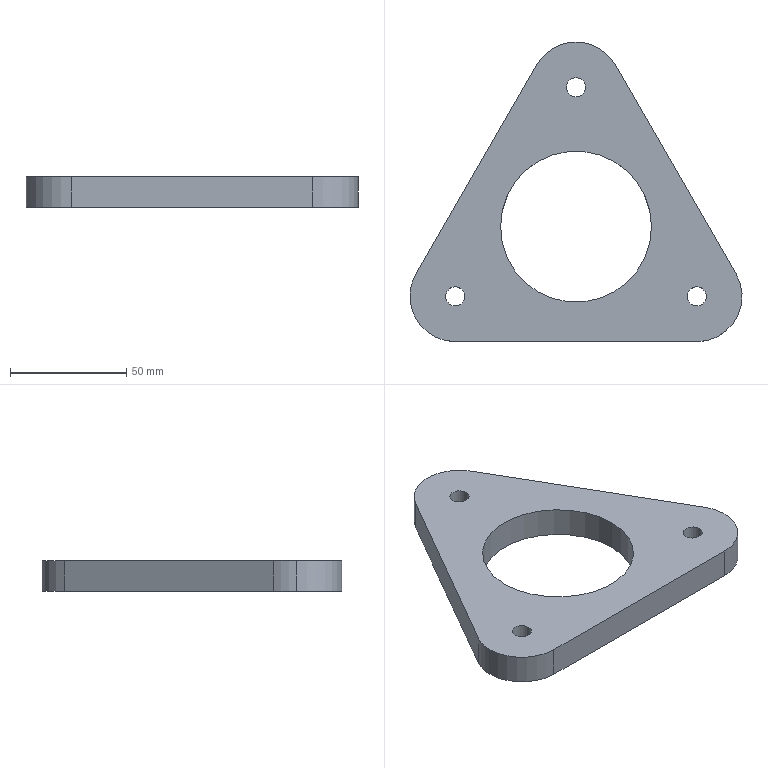Part | SolidWorks | features Extrusion 1, ICE 1, Scale 1 | 1 solid | 36 faces | box 143 x 129.067 x 13 mm | volume 109293 mm3 | cylinder 22 | plane 14 | commonest cylinder face diameters 8.255 x6 11.7 x6 2.6 x4 39 x4 65 x2
STEP:
#1=CARTESIAN_POINT('',(56.847,-26.746,3.9));
#2=VERTEX_POINT('',#1);
#3=CARTESIAN_POINT('',(46.15,-30.022,3.9));
#4=VERTEX_POINT('',#3);
#5=CARTESIAN_POINT('',(52.,-30.022,3.9));
#6=DIRECTION('',(0.,0.,1.));
#7=DIRECTION('',(1.,0.,0.));
#8=AXIS2_PLACEMENT_3D('',#5,#6,#7);
#9=CIRCLE('',#8,5.85);
#10=EDGE_CURVE('',#2,#4,#9,.T.);
#11=ORIENTED_EDGE('',*,*,#10,.T.);
#12=CARTESIAN_POINT('',(46.15,-30.022,0.));
#13=VERTEX_POINT('',#12);
#14=CARTESIAN_POINT('',(46.15,-30.022,3.9));
#15=DIRECTION('',(0.,0.,-1.));
#16=VECTOR('',#15,1000.);
#17=LINE('',#14,#16);
#18=EDGE_CURVE('',#4,#13,#17,.T.);
#19=ORIENTED_EDGE('',*,*,#18,.T.);
#20=CARTESIAN_POINT('',(56.847,-26.746,0.));
#21=VERTEX_POINT('',#20);
#22=CARTESIAN_POINT('',(52.,-30.022,0.));
#23=DIRECTION('',(0.,0.,1.));
#24=DIRECTION('',(1.,0.,0.));
#25=AXIS2_PLACEMENT_3D('',#22,#23,#24);
#26=CIRCLE('',#25,5.85);
#27=EDGE_CURVE('',#21,#13,#26,.T.);
#28=ORIENTED_EDGE('',*,*,#27,.F.);
#29=CARTESIAN_POINT('',(56.847,-26.746,3.9));
#30=DIRECTION('',(0.,0.,-1.));
#31=VECTOR('',#30,1000.);
#32=LINE('',#29,#31);
#33=EDGE_CURVE('',#2,#21,#32,.T.);
#34=ORIENTED_EDGE('',*,*,#33,.F.);
#35=EDGE_LOOP('',(#11,#19,#28,#34));
#36=FACE_OUTER_BOUND('',#35,.T.);
#37=CARTESIAN_POINT('',(52.,-30.022,3.9));
#38=DIRECTION('',(0.,0.,-1.));
#39=DIRECTION('',(-1.,0.,0.));
#40=AXIS2_PLACEMENT_3D('',#37,#38,#39);
#41=CYLINDRICAL_SURFACE('',#40,5.85);
#42=ADVANCED_FACE('',(#36),#41,.F.);
#43=CARTESIAN_POINT('',(-5.85,60.044,3.9));
#44=VERTEX_POINT('',#43);
#45=CARTESIAN_POINT('',(5.85,60.044,3.9));
#46=VERTEX_POINT('',#45);
#47=CARTESIAN_POINT('',(0.,60.044,3.9));
#48=DIRECTION('',(0.,0.,1.));
#49=DIRECTION('',(1.,0.,0.));
#50=AXIS2_PLACEMENT_3D('',#47,#48,#49);
#51=CIRCLE('',#50,5.85);
#52=EDGE_CURVE('',#44,#46,#51,.T.);
#53=ORIENTED_EDGE('',*,*,#52,.T.);
#54=CARTESIAN_POINT('',(5.85,60.044,0.));
#55=VERTEX_POINT('',#54);
#56=CARTESIAN_POINT('',(5.85,60.044,3.9));
#57=DIRECTION('',(0.,0.,-1.));
#58=VECTOR('',#57,1000.);
#59=LINE('',#56,#58);
#60=EDGE_CURVE('',#46,#55,#59,.T.);
#61=ORIENTED_EDGE('',*,*,#60,.T.);
#62=CARTESIAN_POINT('',(-5.85,60.044,0.));
#63=VERTEX_POINT('',#62);
#64=CARTESIAN_POINT('',(0.,60.044,0.));
#65=DIRECTION('',(0.,0.,1.));
#66=DIRECTION('',(1.,0.,0.));
#67=AXIS2_PLACEMENT_3D('',#64,#65,#66);
#68=CIRCLE('',#67,5.85);
#69=EDGE_CURVE('',#63,#55,#68,.T.);
#70=ORIENTED_EDGE('',*,*,#69,.F.);
#71=CARTESIAN_POINT('',(-5.85,60.044,3.9));
#72=DIRECTION('',(0.,0.,-1.));
#73=VECTOR('',#72,1000.);
#74=LINE('',#71,#73);
#75=EDGE_CURVE('',#44,#63,#74,.T.);
#76=ORIENTED_EDGE('',*,*,#75,.F.);
#77=EDGE_LOOP('',(#53,#61,#70,#76));
#78=FACE_OUTER_BOUND('',#77,.T.);
#79=CARTESIAN_POINT('',(0.,60.044,3.9));
#80=DIRECTION('',(0.,0.,-1.));
#81=DIRECTION('',(-1.,0.,0.));
#82=AXIS2_PLACEMENT_3D('',#79,#80,#81);
#83=CYLINDRICAL_SURFACE('',#82,5.85);
#84=ADVANCED_FACE('',(#78),#83,.F.);
#85=CARTESIAN_POINT('',(-5.26,62.604,3.9));
#86=VERTEX_POINT('',#85);
#87=CARTESIAN_POINT('',(0.,60.044,3.9));
#88=DIRECTION('',(0.,0.,1.));
#89=DIRECTION('',(1.,0.,0.));
#90=AXIS2_PLACEMENT_3D('',#87,#88,#89);
#91=CIRCLE('',#90,5.85);
#92=EDGE_CURVE('',#86,#44,#91,.T.);
#93=ORIENTED_EDGE('',*,*,#92,.T.);
#94=ORIENTED_EDGE('',*,*,#75,.T.);
#95=CARTESIAN_POINT('',(-5.26,62.604,0.));
#96=VERTEX_POINT('',#95);
#97=CARTESIAN_POINT('',(0.,60.044,0.));
#98=DIRECTION('',(0.,0.,1.));
#99=DIRECTION('',(1.,0.,0.));
#100=AXIS2_PLACEMENT_3D('',#97,#98,#99);
#101=CIRCLE('',#100,5.85);
#102=EDGE_CURVE('',#96,#63,#101,.T.);
#103=ORIENTED_EDGE('',*,*,#102,.F.);
#104=CARTESIAN_POINT('',(-5.26,62.604,3.9));
#105=DIRECTION('',(0.,0.,-1.));
#106=VECTOR('',#105,1000.);
#107=LINE('',#104,#106);
#108=EDGE_CURVE('',#86,#96,#107,.T.);
#109=ORIENTED_EDGE('',*,*,#108,.F.);
#110=EDGE_LOOP('',(#93,#94,#103,#109));
#111=FACE_OUTER_BOUND('',#110,.T.);
#112=CARTESIAN_POINT('',(0.,60.044,3.9));
#113=DIRECTION('',(0.,0.,-1.));
#114=DIRECTION('',(-1.,0.,0.));
#115=AXIS2_PLACEMENT_3D('',#112,#113,#114);
#116=CYLINDRICAL_SURFACE('',#115,5.85);
#117=ADVANCED_FACE('',(#111),#116,.F.);
#118=CARTESIAN_POINT('',(-62.084,-34.494,3.9));
#119=VERTEX_POINT('',#118);
#120=CARTESIAN_POINT('',(-62.307,-35.222,3.9));
#121=VERTEX_POINT('',#120);
#122=CARTESIAN_POINT('',(-61.007,-35.222,3.9));
#123=DIRECTION('',(0.,0.,1.));
#124=DIRECTION('',(1.,0.,0.));
#125=AXIS2_PLACEMENT_3D('',#122,#123,#124);
#126=CIRCLE('',#125,1.3);
#127=EDGE_CURVE('',#119,#121,#126,.T.);
#128=ORIENTED_EDGE('',*,*,#127,.T.);
#129=CARTESIAN_POINT('',(-62.307,-35.222,0.));
#130=VERTEX_POINT('',#129);
#131=CARTESIAN_POINT('',(-62.307,-35.222,3.9));
#132=DIRECTION('',(0.,0.,-1.));
#133=VECTOR('',#132,1000.);
#134=LINE('',#131,#133);
#135=EDGE_CURVE('',#121,#130,#134,.T.);
#136=ORIENTED_EDGE('',*,*,#135,.T.);
#137=CARTESIAN_POINT('',(-62.084,-34.494,0.));
#138=VERTEX_POINT('',#137);
#139=CARTESIAN_POINT('',(-61.007,-35.222,0.));
#140=DIRECTION('',(0.,0.,1.));
#141=DIRECTION('',(1.,0.,0.));
#142=AXIS2_PLACEMENT_3D('',#139,#140,#141);
#143=CIRCLE('',#142,1.3);
#144=EDGE_CURVE('',#138,#130,#143,.T.);
#145=ORIENTED_EDGE('',*,*,#144,.F.);
#146=CARTESIAN_POINT('',(-62.084,-34.494,3.9));
#147=DIRECTION('',(0.,0.,-1.));
#148=VECTOR('',#147,1000.);
#149=LINE('',#146,#148);
#150=EDGE_CURVE('',#119,#138,#149,.T.);
#151=ORIENTED_EDGE('',*,*,#150,.F.);
#152=EDGE_LOOP('',(#128,#136,#145,#151));
#153=FACE_OUTER_BOUND('',#152,.T.);
#154=CARTESIAN_POINT('',(-61.007,-35.222,3.9));
#155=DIRECTION('',(0.,0.,-1.));
#156=DIRECTION('',(-1.,0.,0.));
#157=AXIS2_PLACEMENT_3D('',#154,#155,#156);
#158=CYLINDRICAL_SURFACE('',#157,1.3);
#159=ADVANCED_FACE('',(#153),#158,.F.);
#160=CARTESIAN_POINT('',(-32.5,0.,13.));
#161=VERTEX_POINT('',#160);
#162=CARTESIAN_POINT('',(32.5,0.,13.));
#163=VERTEX_POINT('',#162);
#164=CARTESIAN_POINT('',(0.,0.,13.));
#165=DIRECTION('',(0.,0.,1.));
#166=DIRECTION('',(1.,0.,0.));
#167=AXIS2_PLACEMENT_3D('',#164,#165,#166);
#168=CIRCLE('',#167,32.5);
#169=EDGE_CURVE('',#161,#163,#168,.T.);
#170=ORIENTED_EDGE('',*,*,#169,.T.);
#171=CARTESIAN_POINT('',(32.5,0.,0.));
#172=VERTEX_POINT('',#171);
#173=CARTESIAN_POINT('',(32.5,0.,13.));
#174=DIRECTION('',(0.,0.,-1.));
#175=VECTOR('',#174,1000.);
#176=LINE('',#173,#175);
#177=EDGE_CURVE('',#163,#172,#176,.T.);
#178=ORIENTED_EDGE('',*,*,#177,.T.);
#179=CARTESIAN_POINT('',(-32.5,0.,0.));
#180=VERTEX_POINT('',#179);
#181=CARTESIAN_POINT('',(0.,0.,0.));
#182=DIRECTION('',(0.,0.,1.));
#183=DIRECTION('',(1.,0.,0.));
#184=AXIS2_PLACEMENT_3D('',#181,#182,#183);
#185=CIRCLE('',#184,32.5);
#186=EDGE_CURVE('',#180,#172,#185,.T.);
#187=ORIENTED_EDGE('',*,*,#186,.F.);
#188=CARTESIAN_POINT('',(-32.5,0.,13.));
#189=DIRECTION('',(0.,0.,-1.));
#190=VECTOR('',#189,1000.);
#191=LINE('',#188,#190);
#192=EDGE_CURVE('',#161,#180,#191,.T.);
#193=ORIENTED_EDGE('',*,*,#192,.F.);
#194=EDGE_LOOP('',(#170,#178,#187,#193));
#195=FACE_OUTER_BOUND('',#194,.T.);
#196=CARTESIAN_POINT('',(0.,0.,13.));
#197=DIRECTION('',(0.,0.,-1.));
#198=DIRECTION('',(-1.,0.,0.));
#199=AXIS2_PLACEMENT_3D('',#196,#197,#198);
#200=CYLINDRICAL_SURFACE('',#199,32.5);
#201=ADVANCED_FACE('',(#195),#200,.F.);
#202=CARTESIAN_POINT('',(-4.127,60.044,13.));
#203=VERTEX_POINT('',#202);
#204=CARTESIAN_POINT('',(4.127,60.044,13.));
#205=VERTEX_POINT('',#204);
#206=CARTESIAN_POINT('',(0.,60.044,13.));
#207=DIRECTION('',(0.,0.,1.));
#208=DIRECTION('',(1.,0.,0.));
#209=AXIS2_PLACEMENT_3D('',#206,#207,#208);
#210=CIRCLE('',#209,4.127);
#211=EDGE_CURVE('',#203,#205,#210,.T.);
#212=ORIENTED_EDGE('',*,*,#211,.T.);
#213=CARTESIAN_POINT('',(4.128,60.044,3.9));
#214=VERTEX_POINT('',#213);
#215=CARTESIAN_POINT('',(4.127,60.044,13.));
#216=DIRECTION('',(0.,0.,-1.));
#217=VECTOR('',#216,1000.);
#218=LINE('',#215,#217);
#219=EDGE_CURVE('',#205,#214,#218,.T.);
#220=ORIENTED_EDGE('',*,*,#219,.T.);
#221=CARTESIAN_POINT('',(-4.127,60.044,3.9));
#222=VERTEX_POINT('',#221);
#223=CARTESIAN_POINT('',(0.,60.044,3.9));
#224=DIRECTION('',(0.,0.,1.));
#225=DIRECTION('',(1.,0.,0.));
#226=AXIS2_PLACEMENT_3D('',#223,#224,#225);
#227=CIRCLE('',#226,4.127);
#228=EDGE_CURVE('',#222,#214,#227,.T.);
#229=ORIENTED_EDGE('',*,*,#228,.F.);
#230=CARTESIAN_POINT('',(-4.127,60.044,13.));
#231=DIRECTION('',(0.,0.,-1.));
#232=VECTOR('',#231,1000.);
#233=LINE('',#230,#232);
#234=EDGE_CURVE('',#203,#222,#233,.T.);
#235=ORIENTED_EDGE('',*,*,#234,.F.);
#236=EDGE_LOOP('',(#212,#220,#229,#235));
#237=FACE_OUTER_BOUND('',#236,.T.);
#238=CARTESIAN_POINT('',(0.,60.044,13.));
#239=DIRECTION('',(0.,0.,-1.));
#240=DIRECTION('',(-1.,0.,0.));
#241=AXIS2_PLACEMENT_3D('',#238,#239,#240);
#242=CYLINDRICAL_SURFACE('',#241,4.127);
#243=ADVANCED_FACE('',(#237),#242,.F.);
#244=CARTESIAN_POINT('',(47.873,-30.022,13.));
#245=VERTEX_POINT('',#244);
#246=CARTESIAN_POINT('',(56.128,-30.022,13.));
#247=VERTEX_POINT('',#246);
#248=CARTESIAN_POINT('',(52.,-30.022,13.));
#249=DIRECTION('',(0.,0.,1.));
#250=DIRECTION('',(1.,0.,0.));
#251=AXIS2_PLACEMENT_3D('',#248,#249,#250);
#252=CIRCLE('',#251,4.127);
#253=EDGE_CURVE('',#245,#247,#252,.T.);
#254=ORIENTED_EDGE('',*,*,#253,.T.);
#255=CARTESIAN_POINT('',(56.127,-30.022,3.9));
#256=VERTEX_POINT('',#255);
#257=CARTESIAN_POINT('',(56.128,-30.022,13.));
#258=DIRECTION('',(0.,0.,-1.));
#259=VECTOR('',#258,1000.);
#260=LINE('',#257,#259);
#261=EDGE_CURVE('',#247,#256,#260,.T.);
#262=ORIENTED_EDGE('',*,*,#261,.T.);
#263=CARTESIAN_POINT('',(47.872,-30.022,3.9));
#264=VERTEX_POINT('',#263);
#265=CARTESIAN_POINT('',(52.,-30.022,3.9));
#266=DIRECTION('',(0.,0.,1.));
#267=DIRECTION('',(1.,0.,0.));
#268=AXIS2_PLACEMENT_3D('',#265,#266,#267);
#269=CIRCLE('',#268,4.127);
#270=EDGE_CURVE('',#264,#256,#269,.T.);
#271=ORIENTED_EDGE('',*,*,#270,.F.);
#272=CARTESIAN_POINT('',(47.873,-30.022,13.));
#273=DIRECTION('',(0.,0.,-1.));
#274=VECTOR('',#273,1000.);
#275=LINE('',#272,#274);
#276=EDGE_CURVE('',#245,#264,#275,.T.);
#277=ORIENTED_EDGE('',*,*,#276,.F.);
#278=EDGE_LOOP('',(#254,#262,#271,#277));
#279=FACE_OUTER_BOUND('',#278,.T.);
#280=CARTESIAN_POINT('',(52.,-30.022,13.));
#281=DIRECTION('',(0.,0.,-1.));
#282=DIRECTION('',(-1.,0.,0.));
#283=AXIS2_PLACEMENT_3D('',#280,#281,#282);
#284=CYLINDRICAL_SURFACE('',#283,4.127);
#285=ADVANCED_FACE('',(#279),#284,.F.);
#286=CARTESIAN_POINT('',(-56.127,-30.022,13.));
#287=VERTEX_POINT('',#286);
#288=CARTESIAN_POINT('',(-47.872,-30.022,13.));
#289=VERTEX_POINT('',#288);
#290=CARTESIAN_POINT('',(-52.,-30.022,13.));
#291=DIRECTION('',(0.,0.,1.));
#292=DIRECTION('',(1.,0.,0.));
#293=AXIS2_PLACEMENT_3D('',#290,#291,#292);
#294=CIRCLE('',#293,4.127);
#295=EDGE_CURVE('',#287,#289,#294,.T.);
#296=ORIENTED_EDGE('',*,*,#295,.T.);
#297=CARTESIAN_POINT('',(-47.872,-30.022,3.9));
#298=VERTEX_POINT('',#297);
#299=CARTESIAN_POINT('',(-47.872,-30.022,13.));
#300=DIRECTION('',(0.,0.,-1.));
#301=VECTOR('',#300,1000.);
#302=LINE('',#299,#301);
#303=EDGE_CURVE('',#289,#298,#302,.T.);
#304=ORIENTED_EDGE('',*,*,#303,.T.);
#305=CARTESIAN_POINT('',(-56.127,-30.022,3.9));
#306=VERTEX_POINT('',#305);
#307=CARTESIAN_POINT('',(-52.,-30.022,3.9));
#308=DIRECTION('',(0.,0.,1.));
#309=DIRECTION('',(1.,0.,0.));
#310=AXIS2_PLACEMENT_3D('',#307,#308,#309);
#311=CIRCLE('',#310,4.127);
#312=EDGE_CURVE('',#306,#298,#311,.T.);
#313=ORIENTED_EDGE('',*,*,#312,.F.);
#314=CARTESIAN_POINT('',(-56.127,-30.022,13.));
#315=DIRECTION('',(0.,0.,-1.));
#316=VECTOR('',#315,1000.);
#317=LINE('',#314,#316);
#318=EDGE_CURVE('',#287,#306,#317,.T.);
#319=ORIENTED_EDGE('',*,*,#318,.F.);
#320=EDGE_LOOP('',(#296,#304,#313,#319));
#321=FACE_OUTER_BOUND('',#320,.T.);
#322=CARTESIAN_POINT('',(-52.,-30.022,13.));
#323=DIRECTION('',(0.,0.,-1.));
#324=DIRECTION('',(-1.,0.,0.));
#325=AXIS2_PLACEMENT_3D('',#322,#323,#324);
#326=CYLINDRICAL_SURFACE('',#325,4.127);
#327=ADVANCED_FACE('',(#321),#326,.F.);
#328=CARTESIAN_POINT('',(-71.5,-30.022,13.));
#329=VERTEX_POINT('',#328);
#330=CARTESIAN_POINT('',(-52.,-49.522,13.));
#331=VERTEX_POINT('',#330);
#332=CARTESIAN_POINT('',(-52.,-30.022,13.));
#333=DIRECTION('',(0.,0.,1.));
#334=DIRECTION('',(1.,0.,0.));
#335=AXIS2_PLACEMENT_3D('',#332,#333,#334);
#336=CIRCLE('',#335,19.5);
#337=EDGE_CURVE('',#329,#331,#336,.T.);
#338=ORIENTED_EDGE('',*,*,#337,.F.);
#339=CARTESIAN_POINT('',(-71.5,-30.022,0.));
#340=VERTEX_POINT('',#339);
#341=CARTESIAN_POINT('',(-71.5,-30.022,13.));
#342=DIRECTION('',(0.,0.,-1.));
#343=VECTOR('',#342,1000.);
#344=LINE('',#341,#343);
#345=EDGE_CURVE('',#329,#340,#344,.T.);
#346=ORIENTED_EDGE('',*,*,#345,.T.);
#347=CARTESIAN_POINT('',(-52.,-49.522,0.));
#348=VERTEX_POINT('',#347);
#349=CARTESIAN_POINT('',(-52.,-30.022,0.));
#350=DIRECTION('',(0.,0.,1.));
#351=DIRECTION('',(1.,0.,0.));
#352=AXIS2_PLACEMENT_3D('',#349,#350,#351);
#353=CIRCLE('',#352,19.5);
#354=EDGE_CURVE('',#340,#348,#353,.T.);
#355=ORIENTED_EDGE('',*,*,#354,.T.);
#356=CARTESIAN_POINT('',(-52.,-49.522,13.));
#357=DIRECTION('',(0.,0.,-1.));
#358=VECTOR('',#357,1000.);
#359=LINE('',#356,#358);
#360=EDGE_CURVE('',#331,#348,#359,.T.);
#361=ORIENTED_EDGE('',*,*,#360,.F.);
#362=EDGE_LOOP('',(#338,#346,#355,#361));
#363=FACE_OUTER_BOUND('',#362,.T.);
#364=CARTESIAN_POINT('',(-52.,-30.022,13.));
#365=DIRECTION('',(0.,0.,-1.));
#366=DIRECTION('',(-1.,0.,0.));
#367=AXIS2_PLACEMENT_3D('',#364,#365,#366);
#368=CYLINDRICAL_SURFACE('',#367,19.5);
#369=ADVANCED_FACE('',(#363),#368,.T.);
#370=ORIENTED_EDGE('',*,*,#102,.T.);
#371=ORIENTED_EDGE('',*,*,#69,.T.);
#372=CARTESIAN_POINT('',(5.26,62.604,0.));
#373=VERTEX_POINT('',#372);
#374=CARTESIAN_POINT('',(0.,60.044,0.));
#375=DIRECTION('',(0.,0.,1.));
#376=DIRECTION('',(1.,0.,0.));
#377=AXIS2_PLACEMENT_3D('',#374,#375,#376);
#378=CIRCLE('',#377,5.85);
#379=EDGE_CURVE('',#55,#373,#378,.T.);
#380=ORIENTED_EDGE('',*,*,#379,.T.);
#381=CARTESIAN_POINT('',(1.169,71.013,0.));
#382=VERTEX_POINT('',#381);
#383=CARTESIAN_POINT('',(5.26,62.604,0.));
#384=DIRECTION('',(-0.4375,0.8992,0.));
#385=VECTOR('',#384,1000.);
#386=LINE('',#383,#385);
#387=EDGE_CURVE('',#373,#382,#386,.T.);
#388=ORIENTED_EDGE('',*,*,#387,.T.);
#389=CARTESIAN_POINT('',(-1.169,71.013,0.));
#390=VERTEX_POINT('',#389);
#391=CARTESIAN_POINT('',(0.,70.444,0.));
#392=DIRECTION('',(0.,0.,1.));
#393=DIRECTION('',(1.,0.,0.));
#394=AXIS2_PLACEMENT_3D('',#391,#392,#393);
#395=CIRCLE('',#394,1.3);
#396=EDGE_CURVE('',#382,#390,#395,.T.);
#397=ORIENTED_EDGE('',*,*,#396,.T.);
#398=CARTESIAN_POINT('',(-5.26,62.604,0.));
#399=DIRECTION('',(-0.4375,-0.8992,0.));
#400=VECTOR('',#399,1000.);
#401=LINE('',#398,#400);
#402=EDGE_CURVE('',#390,#96,#401,.T.);
#403=ORIENTED_EDGE('',*,*,#402,.T.);
#404=EDGE_LOOP('',(#370,#371,#380,#388,#397,#403));
#405=FACE_BOUND('',#404,.T.);
#406=ORIENTED_EDGE('',*,*,#186,.T.);
#407=CARTESIAN_POINT('',(0.,0.,0.));
#408=DIRECTION('',(0.,0.,1.));
#409=DIRECTION('',(1.,0.,0.));
#410=AXIS2_PLACEMENT_3D('',#407,#408,#409);
#411=CIRCLE('',#410,32.5);
#412=EDGE_CURVE('',#172,#180,#411,.T.);
#413=ORIENTED_EDGE('',*,*,#412,.T.);
#414=EDGE_LOOP('',(#406,#413));
#415=FACE_BOUND('',#414,.T.);
#416=CARTESIAN_POINT('',(-68.887,-20.272,0.));
#417=VERTEX_POINT('',#416);
#418=CARTESIAN_POINT('',(-52.,-30.022,0.));
#419=DIRECTION('',(0.,0.,1.));
#420=DIRECTION('',(1.,0.,0.));
#421=AXIS2_PLACEMENT_3D('',#418,#419,#420);
#422=CIRCLE('',#421,19.5);
#423=EDGE_CURVE('',#417,#340,#422,.T.);
#424=ORIENTED_EDGE('',*,*,#423,.F.);
#425=CARTESIAN_POINT('',(-16.887,69.794,0.));
#426=VERTEX_POINT('',#425);
#427=CARTESIAN_POINT('',(-68.887,-20.272,0.));
#428=DIRECTION('',(-0.5,-0.866,0.));
#429=VECTOR('',#428,1000.);
#430=LINE('',#427,#429);
#431=EDGE_CURVE('',#426,#417,#430,.T.);
#432=ORIENTED_EDGE('',*,*,#431,.F.);
#433=CARTESIAN_POINT('',(16.887,69.794,0.));
#434=VERTEX_POINT('',#433);
#435=CARTESIAN_POINT('',(0.,60.044,0.));
#436=DIRECTION('',(0.,0.,1.));
#437=DIRECTION('',(1.,0.,0.));
#438=AXIS2_PLACEMENT_3D('',#435,#436,#437);
#439=CIRCLE('',#438,19.5);
#440=EDGE_CURVE('',#434,#426,#439,.T.);
#441=ORIENTED_EDGE('',*,*,#440,.F.);
#442=CARTESIAN_POINT('',(68.887,-20.272,0.));
#443=VERTEX_POINT('',#442);
#444=CARTESIAN_POINT('',(16.887,69.794,0.));
#445=DIRECTION('',(-0.5,0.866,0.));
#446=VECTOR('',#445,1000.);
#447=LINE('',#444,#446);
#448=EDGE_CURVE('',#443,#434,#447,.T.);
#449=ORIENTED_EDGE('',*,*,#448,.F.);
#450=CARTESIAN_POINT('',(52.,-49.522,0.));
#451=VERTEX_POINT('',#450);
#452=CARTESIAN_POINT('',(52.,-30.022,0.));
#453=DIRECTION('',(0.,0.,1.));
#454=DIRECTION('',(1.,0.,0.));
#455=AXIS2_PLACEMENT_3D('',#452,#453,#454);
#456=CIRCLE('',#455,19.5);
#457=EDGE_CURVE('',#451,#443,#456,.T.);
#458=ORIENTED_EDGE('',*,*,#457,.F.);
#459=CARTESIAN_POINT('',(-52.,-49.522,0.));
#460=DIRECTION('',(1.,0.,0.));
#461=VECTOR('',#460,1000.);
#462=LINE('',#459,#461);
#463=EDGE_CURVE('',#348,#451,#462,.T.);
#464=ORIENTED_EDGE('',*,*,#463,.F.);
#465=ORIENTED_EDGE('',*,*,#354,.F.);
#466=EDGE_LOOP('',(#424,#432,#441,#449,#458,#464,#465));
#467=FACE_OUTER_BOUND('',#466,.T.);
#468=CARTESIAN_POINT('',(-51.586,-35.858,0.));
#469=VERTEX_POINT('',#468);
#470=CARTESIAN_POINT('',(-56.847,-26.746,0.));
#471=VERTEX_POINT('',#470);
#472=CARTESIAN_POINT('',(-52.,-30.022,0.));
#473=DIRECTION('',(0.,0.,1.));
#474=DIRECTION('',(1.,0.,0.));
#475=AXIS2_PLACEMENT_3D('',#472,#473,#474);
#476=CIRCLE('',#475,5.85);
#477=EDGE_CURVE('',#469,#471,#476,.T.);
#478=ORIENTED_EDGE('',*,*,#477,.T.);
#479=CARTESIAN_POINT('',(-56.847,-26.746,0.));
#480=DIRECTION('',(-0.56,-0.8285,0.));
#481=VECTOR('',#480,1000.);
#482=LINE('',#479,#481);
#483=EDGE_CURVE('',#471,#138,#482,.T.);
#484=ORIENTED_EDGE('',*,*,#483,.T.);
#485=ORIENTED_EDGE('',*,*,#144,.T.);
#486=CARTESIAN_POINT('',(-60.915,-36.519,0.));
#487=VERTEX_POINT('',#486);
#488=CARTESIAN_POINT('',(-61.007,-35.222,0.));
#489=DIRECTION('',(0.,0.,1.));
#490=DIRECTION('',(1.,0.,0.));
#491=AXIS2_PLACEMENT_3D('',#488,#489,#490);
#492=CIRCLE('',#491,1.3);
#493=EDGE_CURVE('',#130,#487,#492,.T.);
#494=ORIENTED_EDGE('',*,*,#493,.T.);
#495=CARTESIAN_POINT('',(-51.586,-35.858,0.));
#496=DIRECTION('',(0.9975,0.07072,0.));
#497=VECTOR('',#496,1000.);
#498=LINE('',#495,#497);
#499=EDGE_CURVE('',#487,#469,#498,.T.);
#500=ORIENTED_EDGE('',*,*,#499,.T.);
#501=EDGE_LOOP('',(#478,#484,#485,#494,#500));
#502=FACE_BOUND('',#501,.T.);
#503=ORIENTED_EDGE('',*,*,#27,.T.);
#504=CARTESIAN_POINT('',(51.586,-35.858,0.));
#505=VERTEX_POINT('',#504);
#506=CARTESIAN_POINT('',(52.,-30.022,0.));
#507=DIRECTION('',(0.,0.,1.));
#508=DIRECTION('',(1.,0.,0.));
#509=AXIS2_PLACEMENT_3D('',#506,#507,#508);
#510=CIRCLE('',#509,5.85);
#511=EDGE_CURVE('',#13,#505,#510,.T.);
#512=ORIENTED_EDGE('',*,*,#511,.T.);
#513=CARTESIAN_POINT('',(60.915,-36.519,0.));
#514=VERTEX_POINT('',#513);
#515=CARTESIAN_POINT('',(51.586,-35.858,0.));
#516=DIRECTION('',(0.9975,-0.07072,0.));
#517=VECTOR('',#516,1000.);
#518=LINE('',#515,#517);
#519=EDGE_CURVE('',#505,#514,#518,.T.);
#520=ORIENTED_EDGE('',*,*,#519,.T.);
#521=CARTESIAN_POINT('',(62.084,-34.494,0.));
#522=VERTEX_POINT('',#521);
#523=CARTESIAN_POINT('',(61.007,-35.222,0.));
#524=DIRECTION('',(0.,0.,1.));
#525=DIRECTION('',(1.,0.,0.));
#526=AXIS2_PLACEMENT_3D('',#523,#524,#525);
#527=CIRCLE('',#526,1.3);
#528=EDGE_CURVE('',#514,#522,#527,.T.);
#529=ORIENTED_EDGE('',*,*,#528,.T.);
#530=CARTESIAN_POINT('',(56.847,-26.746,0.));
#531=DIRECTION('',(-0.56,0.8285,0.));
#532=VECTOR('',#531,1000.);
#533=LINE('',#530,#532);
#534=EDGE_CURVE('',#522,#21,#533,.T.);
#535=ORIENTED_EDGE('',*,*,#534,.T.);
#536=EDGE_LOOP('',(#503,#512,#520,#529,#535));
#537=FACE_BOUND('',#536,.T.);
#538=CARTESIAN_POINT('',(-52.,-30.022,0.));
#539=DIRECTION('',(0.,0.,1.));
#540=DIRECTION('',(1.,0.,0.));
#541=AXIS2_PLACEMENT_3D('',#538,#539,#540);
#542=PLANE('',#541);
#543=ADVANCED_FACE('',(#405,#415,#467,#502,#537),#542,.F.);
#544=ORIENTED_EDGE('',*,*,#211,.F.);
#545=CARTESIAN_POINT('',(0.,60.044,13.));
#546=DIRECTION('',(0.,0.,1.));
#547=DIRECTION('',(1.,0.,0.));
#548=AXIS2_PLACEMENT_3D('',#545,#546,#547);
#549=CIRCLE('',#548,4.127);
#550=EDGE_CURVE('',#205,#203,#549,.T.);
#551=ORIENTED_EDGE('',*,*,#550,.F.);
#552=EDGE_LOOP('',(#544,#551));
#553=FACE_BOUND('',#552,.T.);
#554=ORIENTED_EDGE('',*,*,#295,.F.);
#555=CARTESIAN_POINT('',(-52.,-30.022,13.));
#556=DIRECTION('',(0.,0.,1.));
#557=DIRECTION('',(1.,0.,0.));
#558=AXIS2_PLACEMENT_3D('',#555,#556,#557);
#559=CIRCLE('',#558,4.127);
#560=EDGE_CURVE('',#289,#287,#559,.T.);
#561=ORIENTED_EDGE('',*,*,#560,.F.);
#562=EDGE_LOOP('',(#554,#561));
#563=FACE_BOUND('',#562,.T.);
#564=CARTESIAN_POINT('',(-68.887,-20.272,13.));
#565=VERTEX_POINT('',#564);
#566=CARTESIAN_POINT('',(-52.,-30.022,13.));
#567=DIRECTION('',(0.,0.,1.));
#568=DIRECTION('',(1.,0.,0.));
#569=AXIS2_PLACEMENT_3D('',#566,#567,#568);
#570=CIRCLE('',#569,19.5);
#571=EDGE_CURVE('',#565,#329,#570,.T.);
#572=ORIENTED_EDGE('',*,*,#571,.T.);
#573=ORIENTED_EDGE('',*,*,#337,.T.);
#574=CARTESIAN_POINT('',(52.,-49.522,13.));
#575=VERTEX_POINT('',#574);
#576=CARTESIAN_POINT('',(-52.,-49.522,13.));
#577=DIRECTION('',(1.,0.,0.));
#578=VECTOR('',#577,1000.);
#579=LINE('',#576,#578);
#580=EDGE_CURVE('',#331,#575,#579,.T.);
#581=ORIENTED_EDGE('',*,*,#580,.T.);
#582=CARTESIAN_POINT('',(68.887,-20.272,13.));
#583=VERTEX_POINT('',#582);
#584=CARTESIAN_POINT('',(52.,-30.022,13.));
#585=DIRECTION('',(0.,0.,1.));
#586=DIRECTION('',(1.,0.,0.));
#587=AXIS2_PLACEMENT_3D('',#584,#585,#586);
#588=CIRCLE('',#587,19.5);
#589=EDGE_CURVE('',#575,#583,#588,.T.);
#590=ORIENTED_EDGE('',*,*,#589,.T.);
#591=CARTESIAN_POINT('',(16.887,69.794,13.));
#592=VERTEX_POINT('',#591);
#593=CARTESIAN_POINT('',(16.887,69.794,13.));
#594=DIRECTION('',(-0.5,0.866,0.));
#595=VECTOR('',#594,1000.);
#596=LINE('',#593,#595);
#597=EDGE_CURVE('',#583,#592,#596,.T.);
#598=ORIENTED_EDGE('',*,*,#597,.T.);
#599=CARTESIAN_POINT('',(-16.887,69.794,13.));
#600=VERTEX_POINT('',#599);
#601=CARTESIAN_POINT('',(0.,60.044,13.));
#602=DIRECTION('',(0.,0.,1.));
#603=DIRECTION('',(1.,0.,0.));
#604=AXIS2_PLACEMENT_3D('',#601,#602,#603);
#605=CIRCLE('',#604,19.5);
#606=EDGE_CURVE('',#592,#600,#605,.T.);
#607=ORIENTED_EDGE('',*,*,#606,.T.);
#608=CARTESIAN_POINT('',(-68.887,-20.272,13.));
#609=DIRECTION('',(-0.5,-0.866,0.));
#610=VECTOR('',#609,1000.);
#611=LINE('',#608,#610);
#612=EDGE_CURVE('',#600,#565,#611,.T.);
#613=ORIENTED_EDGE('',*,*,#612,.T.);
#614=EDGE_LOOP('',(#572,#573,#581,#590,#598,#607,#613));
#615=FACE_OUTER_BOUND('',#614,.T.);
#616=ORIENTED_EDGE('',*,*,#253,.F.);
#617=CARTESIAN_POINT('',(52.,-30.022,13.));
#618=DIRECTION('',(0.,0.,1.));
#619=DIRECTION('',(1.,0.,0.));
#620=AXIS2_PLACEMENT_3D('',#617,#618,#619);
#621=CIRCLE('',#620,4.127);
#622=EDGE_CURVE('',#247,#245,#621,.T.);
#623=ORIENTED_EDGE('',*,*,#622,.F.);
#624=EDGE_LOOP('',(#616,#623));
#625=FACE_BOUND('',#624,.T.);
#626=ORIENTED_EDGE('',*,*,#169,.F.);
#627=CARTESIAN_POINT('',(0.,0.,13.));
#628=DIRECTION('',(0.,0.,1.));
#629=DIRECTION('',(1.,0.,0.));
#630=AXIS2_PLACEMENT_3D('',#627,#628,#629);
#631=CIRCLE('',#630,32.5);
#632=EDGE_CURVE('',#163,#161,#631,.T.);
#633=ORIENTED_EDGE('',*,*,#632,.F.);
#634=EDGE_LOOP('',(#626,#633));
#635=FACE_BOUND('',#634,.T.);
#636=CARTESIAN_POINT('',(-52.,-30.022,13.));
#637=DIRECTION('',(0.,0.,1.));
#638=DIRECTION('',(1.,0.,0.));
#639=AXIS2_PLACEMENT_3D('',#636,#637,#638);
#640=PLANE('',#639);
#641=ADVANCED_FACE('',(#553,#563,#615,#625,#635),#640,.T.);
#642=ORIENTED_EDGE('',*,*,#345,.F.);
#643=ORIENTED_EDGE('',*,*,#571,.F.);
#644=CARTESIAN_POINT('',(-68.887,-20.272,13.));
#645=DIRECTION('',(0.,0.,-1.));
#646=VECTOR('',#645,1000.);
#647=LINE('',#644,#646);
#648=EDGE_CURVE('',#565,#417,#647,.T.);
#649=ORIENTED_EDGE('',*,*,#648,.T.);
#650=ORIENTED_EDGE('',*,*,#423,.T.);
#651=EDGE_LOOP('',(#642,#643,#649,#650));
#652=FACE_OUTER_BOUND('',#651,.T.);
#653=CARTESIAN_POINT('',(-52.,-30.022,13.));
#654=DIRECTION('',(0.,0.,-1.));
#655=DIRECTION('',(-1.,0.,0.));
#656=AXIS2_PLACEMENT_3D('',#653,#654,#655);
#657=CYLINDRICAL_SURFACE('',#656,19.5);
#658=ADVANCED_FACE('',(#652),#657,.T.);
#659=ORIENTED_EDGE('',*,*,#463,.T.);
#660=CARTESIAN_POINT('',(52.,-49.522,13.));
#661=DIRECTION('',(0.,0.,-1.));
#662=VECTOR('',#661,1000.);
#663=LINE('',#660,#662);
#664=EDGE_CURVE('',#575,#451,#663,.T.);
#665=ORIENTED_EDGE('',*,*,#664,.F.);
#666=ORIENTED_EDGE('',*,*,#580,.F.);
#667=ORIENTED_EDGE('',*,*,#360,.T.);
#668=EDGE_LOOP('',(#659,#665,#666,#667));
#669=FACE_OUTER_BOUND('',#668,.T.);
#670=CARTESIAN_POINT('',(-52.,-49.522,13.));
#671=DIRECTION('',(0.,1.,0.));
#672=DIRECTION('',(-1.,0.,0.));
#673=AXIS2_PLACEMENT_3D('',#670,#671,#672);
#674=PLANE('',#673);
#675=ADVANCED_FACE('',(#669),#674,.F.);
#676=ORIENTED_EDGE('',*,*,#457,.T.);
#677=CARTESIAN_POINT('',(68.887,-20.272,13.));
#678=DIRECTION('',(0.,0.,-1.));
#679=VECTOR('',#678,1000.);
#680=LINE('',#677,#679);
#681=EDGE_CURVE('',#583,#443,#680,.T.);
#682=ORIENTED_EDGE('',*,*,#681,.F.);
#683=ORIENTED_EDGE('',*,*,#589,.F.);
#684=ORIENTED_EDGE('',*,*,#664,.T.);
#685=EDGE_LOOP('',(#676,#682,#683,#684));
#686=FACE_OUTER_BOUND('',#685,.T.);
#687=CARTESIAN_POINT('',(52.,-30.022,13.));
#688=DIRECTION('',(0.,0.,-1.));
#689=DIRECTION('',(-1.,0.,0.));
#690=AXIS2_PLACEMENT_3D('',#687,#688,#689);
#691=CYLINDRICAL_SURFACE('',#690,19.5);
#692=ADVANCED_FACE('',(#686),#691,.T.);
#693=ORIENTED_EDGE('',*,*,#448,.T.);
#694=CARTESIAN_POINT('',(16.887,69.794,13.));
#695=DIRECTION('',(0.,0.,-1.));
#696=VECTOR('',#695,1000.);
#697=LINE('',#694,#696);
#698=EDGE_CURVE('',#592,#434,#697,.T.);
#699=ORIENTED_EDGE('',*,*,#698,.F.);
#700=ORIENTED_EDGE('',*,*,#597,.F.);
#701=ORIENTED_EDGE('',*,*,#681,.T.);
#702=EDGE_LOOP('',(#693,#699,#700,#701));
#703=FACE_OUTER_BOUND('',#702,.T.);
#704=CARTESIAN_POINT('',(16.887,69.794,13.));
#705=DIRECTION('',(-0.866,-0.5,0.));
#706=DIRECTION('',(0.5,-0.866,0.));
#707=AXIS2_PLACEMENT_3D('',#704,#705,#706);
#708=PLANE('',#707);
#709=ADVANCED_FACE('',(#703),#708,.F.);
#710=ORIENTED_EDGE('',*,*,#440,.T.);
#711=CARTESIAN_POINT('',(-16.887,69.794,13.));
#712=DIRECTION('',(0.,0.,-1.));
#713=VECTOR('',#712,1000.);
#714=LINE('',#711,#713);
#715=EDGE_CURVE('',#600,#426,#714,.T.);
#716=ORIENTED_EDGE('',*,*,#715,.F.);
#717=ORIENTED_EDGE('',*,*,#606,.F.);
#718=ORIENTED_EDGE('',*,*,#698,.T.);
#719=EDGE_LOOP('',(#710,#716,#717,#718));
#720=FACE_OUTER_BOUND('',#719,.T.);
#721=CARTESIAN_POINT('',(0.,60.044,13.));
#722=DIRECTION('',(0.,0.,-1.));
#723=DIRECTION('',(-1.,0.,0.));
#724=AXIS2_PLACEMENT_3D('',#721,#722,#723);
#725=CYLINDRICAL_SURFACE('',#724,19.5);
#726=ADVANCED_FACE('',(#720),#725,.T.);
#727=ORIENTED_EDGE('',*,*,#431,.T.);
#728=ORIENTED_EDGE('',*,*,#648,.F.);
#729=ORIENTED_EDGE('',*,*,#612,.F.);
#730=ORIENTED_EDGE('',*,*,#715,.T.);
#731=EDGE_LOOP('',(#727,#728,#729,#730));
#732=FACE_OUTER_BOUND('',#731,.T.);
#733=CARTESIAN_POINT('',(-68.887,-20.272,13.));
#734=DIRECTION('',(0.866,-0.5,0.));
#735=DIRECTION('',(0.5,0.866,0.));
#736=AXIS2_PLACEMENT_3D('',#733,#734,#735);
#737=PLANE('',#736);
#738=ADVANCED_FACE('',(#732),#737,.F.);
#739=ORIENTED_EDGE('',*,*,#303,.F.);
#740=ORIENTED_EDGE('',*,*,#560,.T.);
#741=ORIENTED_EDGE('',*,*,#318,.T.);
#742=CARTESIAN_POINT('',(-52.,-30.022,3.9));
#743=DIRECTION('',(0.,0.,1.));
#744=DIRECTION('',(1.,0.,0.));
#745=AXIS2_PLACEMENT_3D('',#742,#743,#744);
#746=CIRCLE('',#745,4.127);
#747=EDGE_CURVE('',#298,#306,#746,.T.);
#748=ORIENTED_EDGE('',*,*,#747,.F.);
#749=EDGE_LOOP('',(#739,#740,#741,#748));
#750=FACE_OUTER_BOUND('',#749,.T.);
#751=CARTESIAN_POINT('',(-52.,-30.022,13.));
#752=DIRECTION('',(0.,0.,-1.));
#753=DIRECTION('',(-1.,0.,0.));
#754=AXIS2_PLACEMENT_3D('',#751,#752,#753);
#755=CYLINDRICAL_SURFACE('',#754,4.127);
#756=ADVANCED_FACE('',(#750),#755,.F.);
#757=ORIENTED_EDGE('',*,*,#261,.F.);
#758=ORIENTED_EDGE('',*,*,#622,.T.);
#759=ORIENTED_EDGE('',*,*,#276,.T.);
#760=CARTESIAN_POINT('',(52.,-30.022,3.9));
#761=DIRECTION('',(0.,0.,1.));
#762=DIRECTION('',(1.,0.,0.));
#763=AXIS2_PLACEMENT_3D('',#760,#761,#762);
#764=CIRCLE('',#763,4.127);
#765=EDGE_CURVE('',#256,#264,#764,.T.);
#766=ORIENTED_EDGE('',*,*,#765,.F.);
#767=EDGE_LOOP('',(#757,#758,#759,#766));
#768=FACE_OUTER_BOUND('',#767,.T.);
#769=CARTESIAN_POINT('',(52.,-30.022,13.));
#770=DIRECTION('',(0.,0.,-1.));
#771=DIRECTION('',(-1.,0.,0.));
#772=AXIS2_PLACEMENT_3D('',#769,#770,#771);
#773=CYLINDRICAL_SURFACE('',#772,4.127);
#774=ADVANCED_FACE('',(#768),#773,.F.);
#775=ORIENTED_EDGE('',*,*,#219,.F.);
#776=ORIENTED_EDGE('',*,*,#550,.T.);
#777=ORIENTED_EDGE('',*,*,#234,.T.);
#778=CARTESIAN_POINT('',(0.,60.044,3.9));
#779=DIRECTION('',(0.,0.,1.));
#780=DIRECTION('',(1.,0.,0.));
#781=AXIS2_PLACEMENT_3D('',#778,#779,#780);
#782=CIRCLE('',#781,4.127);
#783=EDGE_CURVE('',#214,#222,#782,.T.);
#784=ORIENTED_EDGE('',*,*,#783,.F.);
#785=EDGE_LOOP('',(#775,#776,#777,#784));
#786=FACE_OUTER_BOUND('',#785,.T.);
#787=CARTESIAN_POINT('',(0.,60.044,13.));
#788=DIRECTION('',(0.,0.,-1.));
#789=DIRECTION('',(-1.,0.,0.));
#790=AXIS2_PLACEMENT_3D('',#787,#788,#789);
#791=CYLINDRICAL_SURFACE('',#790,4.127);
#792=ADVANCED_FACE('',(#786),#791,.F.);
#793=ORIENTED_EDGE('',*,*,#177,.F.);
#794=ORIENTED_EDGE('',*,*,#632,.T.);
#795=ORIENTED_EDGE('',*,*,#192,.T.);
#796=ORIENTED_EDGE('',*,*,#412,.F.);
#797=EDGE_LOOP('',(#793,#794,#795,#796));
#798=FACE_OUTER_BOUND('',#797,.T.);
#799=CARTESIAN_POINT('',(0.,0.,13.));
#800=DIRECTION('',(0.,0.,-1.));
#801=DIRECTION('',(-1.,0.,0.));
#802=AXIS2_PLACEMENT_3D('',#799,#800,#801);
#803=CYLINDRICAL_SURFACE('',#802,32.5);
#804=ADVANCED_FACE('',(#798),#803,.F.);
#805=CARTESIAN_POINT('',(-51.586,-35.858,3.9));
#806=VERTEX_POINT('',#805);
#807=CARTESIAN_POINT('',(-56.847,-26.746,3.9));
#808=VERTEX_POINT('',#807);
#809=CARTESIAN_POINT('',(-52.,-30.022,3.9));
#810=DIRECTION('',(0.,0.,1.));
#811=DIRECTION('',(1.,0.,0.));
#812=AXIS2_PLACEMENT_3D('',#809,#810,#811);
#813=CIRCLE('',#812,5.85);
#814=EDGE_CURVE('',#806,#808,#813,.T.);
#815=ORIENTED_EDGE('',*,*,#814,.F.);
#816=CARTESIAN_POINT('',(-60.915,-36.519,3.9));
#817=VERTEX_POINT('',#816);
#818=CARTESIAN_POINT('',(-51.586,-35.858,3.9));
#819=DIRECTION('',(0.9975,0.07072,0.));
#820=VECTOR('',#819,1000.);
#821=LINE('',#818,#820);
#822=EDGE_CURVE('',#817,#806,#821,.T.);
#823=ORIENTED_EDGE('',*,*,#822,.F.);
#824=CARTESIAN_POINT('',(-61.007,-35.222,3.9));
#825=DIRECTION('',(0.,0.,1.));
#826=DIRECTION('',(1.,0.,0.));
#827=AXIS2_PLACEMENT_3D('',#824,#825,#826);
#828=CIRCLE('',#827,1.3);
#829=EDGE_CURVE('',#121,#817,#828,.T.);
#830=ORIENTED_EDGE('',*,*,#829,.F.);
#831=ORIENTED_EDGE('',*,*,#127,.F.);
#832=CARTESIAN_POINT('',(-56.847,-26.746,3.9));
#833=DIRECTION('',(-0.56,-0.8285,0.));
#834=VECTOR('',#833,1000.);
#835=LINE('',#832,#834);
#836=EDGE_CURVE('',#808,#119,#835,.T.);
#837=ORIENTED_EDGE('',*,*,#836,.F.);
#838=EDGE_LOOP('',(#815,#823,#830,#831,#837));
#839=FACE_OUTER_BOUND('',#838,.T.);
#840=ORIENTED_EDGE('',*,*,#312,.T.);
#841=ORIENTED_EDGE('',*,*,#747,.T.);
#842=EDGE_LOOP('',(#840,#841));
#843=FACE_BOUND('',#842,.T.);
#844=CARTESIAN_POINT('',(-52.,-30.022,3.9));
#845=DIRECTION('',(0.,0.,1.));
#846=DIRECTION('',(1.,0.,0.));
#847=AXIS2_PLACEMENT_3D('',#844,#845,#846);
#848=PLANE('',#847);
#849=ADVANCED_FACE('',(#839,#843),#848,.F.);
#850=ORIENTED_EDGE('',*,*,#477,.F.);
#851=CARTESIAN_POINT('',(-51.586,-35.858,3.9));
#852=DIRECTION('',(0.,0.,-1.));
#853=VECTOR('',#852,1000.);
#854=LINE('',#851,#853);
#855=EDGE_CURVE('',#806,#469,#854,.T.);
#856=ORIENTED_EDGE('',*,*,#855,.F.);
#857=ORIENTED_EDGE('',*,*,#814,.T.);
#858=CARTESIAN_POINT('',(-56.847,-26.746,3.9));
#859=DIRECTION('',(0.,0.,-1.));
#860=VECTOR('',#859,1000.);
#861=LINE('',#858,#860);
#862=EDGE_CURVE('',#808,#471,#861,.T.);
#863=ORIENTED_EDGE('',*,*,#862,.T.);
#864=EDGE_LOOP('',(#850,#856,#857,#863));
#865=FACE_OUTER_BOUND('',#864,.T.);
#866=CARTESIAN_POINT('',(-52.,-30.022,3.9));
#867=DIRECTION('',(0.,0.,-1.));
#868=DIRECTION('',(-1.,0.,0.));
#869=AXIS2_PLACEMENT_3D('',#866,#867,#868);
#870=CYLINDRICAL_SURFACE('',#869,5.85);
#871=ADVANCED_FACE('',(#865),#870,.F.);
#872=ORIENTED_EDGE('',*,*,#483,.F.);
#873=ORIENTED_EDGE('',*,*,#862,.F.);
#874=ORIENTED_EDGE('',*,*,#836,.T.);
#875=ORIENTED_EDGE('',*,*,#150,.T.);
#876=EDGE_LOOP('',(#872,#873,#874,#875));
#877=FACE_OUTER_BOUND('',#876,.T.);
#878=CARTESIAN_POINT('',(-56.847,-26.746,3.9));
#879=DIRECTION('',(0.8285,-0.56,0.));
#880=DIRECTION('',(0.56,0.8285,0.));
#881=AXIS2_PLACEMENT_3D('',#878,#879,#880);
#882=PLANE('',#881);
#883=ADVANCED_FACE('',(#877),#882,.T.);
#884=ORIENTED_EDGE('',*,*,#135,.F.);
#885=ORIENTED_EDGE('',*,*,#829,.T.);
#886=CARTESIAN_POINT('',(-60.915,-36.519,3.9));
#887=DIRECTION('',(0.,0.,-1.));
#888=VECTOR('',#887,1000.);
#889=LINE('',#886,#888);
#890=EDGE_CURVE('',#817,#487,#889,.T.);
#891=ORIENTED_EDGE('',*,*,#890,.T.);
#892=ORIENTED_EDGE('',*,*,#493,.F.);
#893=EDGE_LOOP('',(#884,#885,#891,#892));
#894=FACE_OUTER_BOUND('',#893,.T.);
#895=CARTESIAN_POINT('',(-61.007,-35.222,3.9));
#896=DIRECTION('',(0.,0.,-1.));
#897=DIRECTION('',(-1.,0.,0.));
#898=AXIS2_PLACEMENT_3D('',#895,#896,#897);
#899=CYLINDRICAL_SURFACE('',#898,1.3);
#900=ADVANCED_FACE('',(#894),#899,.F.);
#901=ORIENTED_EDGE('',*,*,#499,.F.);
#902=ORIENTED_EDGE('',*,*,#890,.F.);
#903=ORIENTED_EDGE('',*,*,#822,.T.);
#904=ORIENTED_EDGE('',*,*,#855,.T.);
#905=EDGE_LOOP('',(#901,#902,#903,#904));
#906=FACE_OUTER_BOUND('',#905,.T.);
#907=CARTESIAN_POINT('',(-51.586,-35.858,3.9));
#908=DIRECTION('',(-0.07072,0.9975,0.));
#909=DIRECTION('',(-0.9975,-0.07072,0.));
#910=AXIS2_PLACEMENT_3D('',#907,#908,#909);
#911=PLANE('',#910);
#912=ADVANCED_FACE('',(#906),#911,.T.);
#913=ORIENTED_EDGE('',*,*,#92,.F.);
#914=CARTESIAN_POINT('',(-1.169,71.013,3.9));
#915=VERTEX_POINT('',#914);
#916=CARTESIAN_POINT('',(-5.26,62.604,3.9));
#917=DIRECTION('',(-0.4375,-0.8992,0.));
#918=VECTOR('',#917,1000.);
#919=LINE('',#916,#918);
#920=EDGE_CURVE('',#915,#86,#919,.T.);
#921=ORIENTED_EDGE('',*,*,#920,.F.);
#922=CARTESIAN_POINT('',(1.169,71.013,3.9));
#923=VERTEX_POINT('',#922);
#924=CARTESIAN_POINT('',(0.,70.444,3.9));
#925=DIRECTION('',(0.,0.,1.));
#926=DIRECTION('',(1.,0.,0.));
#927=AXIS2_PLACEMENT_3D('',#924,#925,#926);
#928=CIRCLE('',#927,1.3);
#929=EDGE_CURVE('',#923,#915,#928,.T.);
#930=ORIENTED_EDGE('',*,*,#929,.F.);
#931=CARTESIAN_POINT('',(5.26,62.604,3.9));
#932=VERTEX_POINT('',#931);
#933=CARTESIAN_POINT('',(5.26,62.604,3.9));
#934=DIRECTION('',(-0.4375,0.8992,0.));
#935=VECTOR('',#934,1000.);
#936=LINE('',#933,#935);
#937=EDGE_CURVE('',#932,#923,#936,.T.);
#938=ORIENTED_EDGE('',*,*,#937,.F.);
#939=CARTESIAN_POINT('',(0.,60.044,3.9));
#940=DIRECTION('',(0.,0.,1.));
#941=DIRECTION('',(1.,0.,0.));
#942=AXIS2_PLACEMENT_3D('',#939,#940,#941);
#943=CIRCLE('',#942,5.85);
#944=EDGE_CURVE('',#46,#932,#943,.T.);
#945=ORIENTED_EDGE('',*,*,#944,.F.);
#946=ORIENTED_EDGE('',*,*,#52,.F.);
#947=EDGE_LOOP('',(#913,#921,#930,#938,#945,#946));
#948=FACE_OUTER_BOUND('',#947,.T.);
#949=ORIENTED_EDGE('',*,*,#228,.T.);
#950=ORIENTED_EDGE('',*,*,#783,.T.);
#951=EDGE_LOOP('',(#949,#950));
#952=FACE_BOUND('',#951,.T.);
#953=CARTESIAN_POINT('',(0.,60.044,3.9));
#954=DIRECTION('',(0.,0.,1.));
#955=DIRECTION('',(1.,0.,0.));
#956=AXIS2_PLACEMENT_3D('',#953,#954,#955);
#957=PLANE('',#956);
#958=ADVANCED_FACE('',(#948,#952),#957,.F.);
#959=ORIENTED_EDGE('',*,*,#60,.F.);
#960=ORIENTED_EDGE('',*,*,#944,.T.);
#961=CARTESIAN_POINT('',(5.26,62.604,3.9));
#962=DIRECTION('',(0.,0.,-1.));
#963=VECTOR('',#962,1000.);
#964=LINE('',#961,#963);
#965=EDGE_CURVE('',#932,#373,#964,.T.);
#966=ORIENTED_EDGE('',*,*,#965,.T.);
#967=ORIENTED_EDGE('',*,*,#379,.F.);
#968=EDGE_LOOP('',(#959,#960,#966,#967));
#969=FACE_OUTER_BOUND('',#968,.T.);
#970=CARTESIAN_POINT('',(0.,60.044,3.9));
#971=DIRECTION('',(0.,0.,-1.));
#972=DIRECTION('',(-1.,0.,0.));
#973=AXIS2_PLACEMENT_3D('',#970,#971,#972);
#974=CYLINDRICAL_SURFACE('',#973,5.85);
#975=ADVANCED_FACE('',(#969),#974,.F.);
#976=ORIENTED_EDGE('',*,*,#387,.F.);
#977=ORIENTED_EDGE('',*,*,#965,.F.);
#978=ORIENTED_EDGE('',*,*,#937,.T.);
#979=CARTESIAN_POINT('',(1.169,71.013,3.9));
#980=DIRECTION('',(0.,0.,-1.));
#981=VECTOR('',#980,1000.);
#982=LINE('',#979,#981);
#983=EDGE_CURVE('',#923,#382,#982,.T.);
#984=ORIENTED_EDGE('',*,*,#983,.T.);
#985=EDGE_LOOP('',(#976,#977,#978,#984));
#986=FACE_OUTER_BOUND('',#985,.T.);
#987=CARTESIAN_POINT('',(5.26,62.604,3.9));
#988=DIRECTION('',(-0.8992,-0.4375,0.));
#989=DIRECTION('',(0.4375,-0.8992,0.));
#990=AXIS2_PLACEMENT_3D('',#987,#988,#989);
#991=PLANE('',#990);
#992=ADVANCED_FACE('',(#986),#991,.T.);
#993=ORIENTED_EDGE('',*,*,#396,.F.);
#994=ORIENTED_EDGE('',*,*,#983,.F.);
#995=ORIENTED_EDGE('',*,*,#929,.T.);
#996=CARTESIAN_POINT('',(-1.169,71.013,3.9));
#997=DIRECTION('',(0.,0.,-1.));
#998=VECTOR('',#997,1000.);
#999=LINE('',#996,#998);
#1000=EDGE_CURVE('',#915,#390,#999,.T.);
#1001=ORIENTED_EDGE('',*,*,#1000,.T.);
#1002=EDGE_LOOP('',(#993,#994,#995,#1001));
#1003=FACE_OUTER_BOUND('',#1002,.T.);
#1004=CARTESIAN_POINT('',(0.,70.444,3.9));
#1005=DIRECTION('',(0.,0.,-1.));
#1006=DIRECTION('',(-1.,0.,0.));
#1007=AXIS2_PLACEMENT_3D('',#1004,#1005,#1006);
#1008=CYLINDRICAL_SURFACE('',#1007,1.3);
#1009=ADVANCED_FACE('',(#1003),#1008,.F.);
#1010=ORIENTED_EDGE('',*,*,#402,.F.);
#1011=ORIENTED_EDGE('',*,*,#1000,.F.);
#1012=ORIENTED_EDGE('',*,*,#920,.T.);
#1013=ORIENTED_EDGE('',*,*,#108,.T.);
#1014=EDGE_LOOP('',(#1010,#1011,#1012,#1013));
#1015=FACE_OUTER_BOUND('',#1014,.T.);
#1016=CARTESIAN_POINT('',(-5.26,62.604,3.9));
#1017=DIRECTION('',(0.8992,-0.4375,0.));
#1018=DIRECTION('',(0.4375,0.8992,0.));
#1019=AXIS2_PLACEMENT_3D('',#1016,#1017,#1018);
#1020=PLANE('',#1019);
#1021=ADVANCED_FACE('',(#1015),#1020,.T.);
#1022=ORIENTED_EDGE('',*,*,#10,.F.);
#1023=CARTESIAN_POINT('',(62.084,-34.494,3.9));
#1024=VERTEX_POINT('',#1023);
#1025=CARTESIAN_POINT('',(56.847,-26.746,3.9));
#1026=DIRECTION('',(-0.56,0.8285,0.));
#1027=VECTOR('',#1026,1000.);
#1028=LINE('',#1025,#1027);
#1029=EDGE_CURVE('',#1024,#2,#1028,.T.);
#1030=ORIENTED_EDGE('',*,*,#1029,.F.);
#1031=CARTESIAN_POINT('',(60.915,-36.519,3.9));
#1032=VERTEX_POINT('',#1031);
#1033=CARTESIAN_POINT('',(61.007,-35.222,3.9));
#1034=DIRECTION('',(0.,0.,1.));
#1035=DIRECTION('',(1.,0.,0.));
#1036=AXIS2_PLACEMENT_3D('',#1033,#1034,#1035);
#1037=CIRCLE('',#1036,1.3);
#1038=EDGE_CURVE('',#1032,#1024,#1037,.T.);
#1039=ORIENTED_EDGE('',*,*,#1038,.F.);
#1040=CARTESIAN_POINT('',(51.586,-35.858,3.9));
#1041=VERTEX_POINT('',#1040);
#1042=CARTESIAN_POINT('',(51.586,-35.858,3.9));
#1043=DIRECTION('',(0.9975,-0.07072,0.));
#1044=VECTOR('',#1043,1000.);
#1045=LINE('',#1042,#1044);
#1046=EDGE_CURVE('',#1041,#1032,#1045,.T.);
#1047=ORIENTED_EDGE('',*,*,#1046,.F.);
#1048=CARTESIAN_POINT('',(52.,-30.022,3.9));
#1049=DIRECTION('',(0.,0.,1.));
#1050=DIRECTION('',(1.,0.,0.));
#1051=AXIS2_PLACEMENT_3D('',#1048,#1049,#1050);
#1052=CIRCLE('',#1051,5.85);
#1053=EDGE_CURVE('',#4,#1041,#1052,.T.);
#1054=ORIENTED_EDGE('',*,*,#1053,.F.);
#1055=EDGE_LOOP('',(#1022,#1030,#1039,#1047,#1054));
#1056=FACE_OUTER_BOUND('',#1055,.T.);
#1057=ORIENTED_EDGE('',*,*,#270,.T.);
#1058=ORIENTED_EDGE('',*,*,#765,.T.);
#1059=EDGE_LOOP('',(#1057,#1058));
#1060=FACE_BOUND('',#1059,.T.);
#1061=CARTESIAN_POINT('',(52.,-30.022,3.9));
#1062=DIRECTION('',(0.,0.,1.));
#1063=DIRECTION('',(1.,0.,0.));
#1064=AXIS2_PLACEMENT_3D('',#1061,#1062,#1063);
#1065=PLANE('',#1064);
#1066=ADVANCED_FACE('',(#1056,#1060),#1065,.F.);
#1067=ORIENTED_EDGE('',*,*,#18,.F.);
#1068=ORIENTED_EDGE('',*,*,#1053,.T.);
#1069=CARTESIAN_POINT('',(51.586,-35.858,3.9));
#1070=DIRECTION('',(0.,0.,-1.));
#1071=VECTOR('',#1070,1000.);
#1072=LINE('',#1069,#1071);
#1073=EDGE_CURVE('',#1041,#505,#1072,.T.);
#1074=ORIENTED_EDGE('',*,*,#1073,.T.);
#1075=ORIENTED_EDGE('',*,*,#511,.F.);
#1076=EDGE_LOOP('',(#1067,#1068,#1074,#1075));
#1077=FACE_OUTER_BOUND('',#1076,.T.);
#1078=CARTESIAN_POINT('',(52.,-30.022,3.9));
#1079=DIRECTION('',(0.,0.,-1.));
#1080=DIRECTION('',(-1.,0.,0.));
#1081=AXIS2_PLACEMENT_3D('',#1078,#1079,#1080);
#1082=CYLINDRICAL_SURFACE('',#1081,5.85);
#1083=ADVANCED_FACE('',(#1077),#1082,.F.);
#1084=ORIENTED_EDGE('',*,*,#519,.F.);
#1085=ORIENTED_EDGE('',*,*,#1073,.F.);
#1086=ORIENTED_EDGE('',*,*,#1046,.T.);
#1087=CARTESIAN_POINT('',(60.915,-36.519,3.9));
#1088=DIRECTION('',(0.,0.,-1.));
#1089=VECTOR('',#1088,1000.);
#1090=LINE('',#1087,#1089);
#1091=EDGE_CURVE('',#1032,#514,#1090,.T.);
#1092=ORIENTED_EDGE('',*,*,#1091,.T.);
#1093=EDGE_LOOP('',(#1084,#1085,#1086,#1092));
#1094=FACE_OUTER_BOUND('',#1093,.T.);
#1095=CARTESIAN_POINT('',(51.586,-35.858,3.9));
#1096=DIRECTION('',(0.07072,0.9975,0.));
#1097=DIRECTION('',(-0.9975,0.07072,0.));
#1098=AXIS2_PLACEMENT_3D('',#1095,#1096,#1097);
#1099=PLANE('',#1098);
#1100=ADVANCED_FACE('',(#1094),#1099,.T.);
#1101=ORIENTED_EDGE('',*,*,#528,.F.);
#1102=ORIENTED_EDGE('',*,*,#1091,.F.);
#1103=ORIENTED_EDGE('',*,*,#1038,.T.);
#1104=CARTESIAN_POINT('',(62.084,-34.494,3.9));
#1105=DIRECTION('',(0.,0.,-1.));
#1106=VECTOR('',#1105,1000.);
#1107=LINE('',#1104,#1106);
#1108=EDGE_CURVE('',#1024,#522,#1107,.T.);
#1109=ORIENTED_EDGE('',*,*,#1108,.T.);
#1110=EDGE_LOOP('',(#1101,#1102,#1103,#1109));
#1111=FACE_OUTER_BOUND('',#1110,.T.);
#1112=CARTESIAN_POINT('',(61.007,-35.222,3.9));
#1113=DIRECTION('',(0.,0.,-1.));
#1114=DIRECTION('',(-1.,0.,0.));
#1115=AXIS2_PLACEMENT_3D('',#1112,#1113,#1114);
#1116=CYLINDRICAL_SURFACE('',#1115,1.3);
#1117=ADVANCED_FACE('',(#1111),#1116,.F.);
#1118=ORIENTED_EDGE('',*,*,#534,.F.);
#1119=ORIENTED_EDGE('',*,*,#1108,.F.);
#1120=ORIENTED_EDGE('',*,*,#1029,.T.);
#1121=ORIENTED_EDGE('',*,*,#33,.T.);
#1122=EDGE_LOOP('',(#1118,#1119,#1120,#1121));
#1123=FACE_OUTER_BOUND('',#1122,.T.);
#1124=CARTESIAN_POINT('',(56.847,-26.746,3.9));
#1125=DIRECTION('',(-0.8285,-0.56,0.));
#1126=DIRECTION('',(0.56,-0.8285,0.));
#1127=AXIS2_PLACEMENT_3D('',#1124,#1125,#1126);
#1128=PLANE('',#1127);
#1129=ADVANCED_FACE('',(#1123),#1128,.T.);
#1130=CLOSED_SHELL('',(#42,#84,#117,#159,#201,#243,#285,#327,#369,#543,#641,#658,#675,#692,#709,#726,#738,#756,#774,#792,#804,#849,#871,#883,#900,#912,#958,#975,#992,#1009,#1021,#1066,#1083,#1100,#1117,#1129));
#1131=MANIFOLD_SOLID_BREP('',#1130);
#1132=CARTESIAN_POINT('',(0.,0.,0.));
#1133=DIRECTION('',(0.,0.,1.));
#1134=DIRECTION('',(1.,0.,0.));
#1135=AXIS2_PLACEMENT_3D('',#1132,#1133,#1134);
#1136=(LENGTH_UNIT()NAMED_UNIT(*)SI_UNIT(.MILLI.,.METRE.));
#1137=UNCERTAINTY_MEASURE_WITH_UNIT(LENGTH_MEASURE(0.00001),#1136,'','');
#1138=(NAMED_UNIT(*)PLANE_ANGLE_UNIT()SI_UNIT($,.RADIAN.));
#1139=(NAMED_UNIT(*)SI_UNIT($,.STERADIAN.)SOLID_ANGLE_UNIT());
#1140=(GEOMETRIC_REPRESENTATION_CONTEXT(3)GLOBAL_UNCERTAINTY_ASSIGNED_CONTEXT((#1137))GLOBAL_UNIT_ASSIGNED_CONTEXT((#1136,#1138,#1139))REPRESENTATION_CONTEXT('',''));
#1141=ADVANCED_BREP_SHAPE_REPRESENTATION('',(#1131,#1135),#1140);